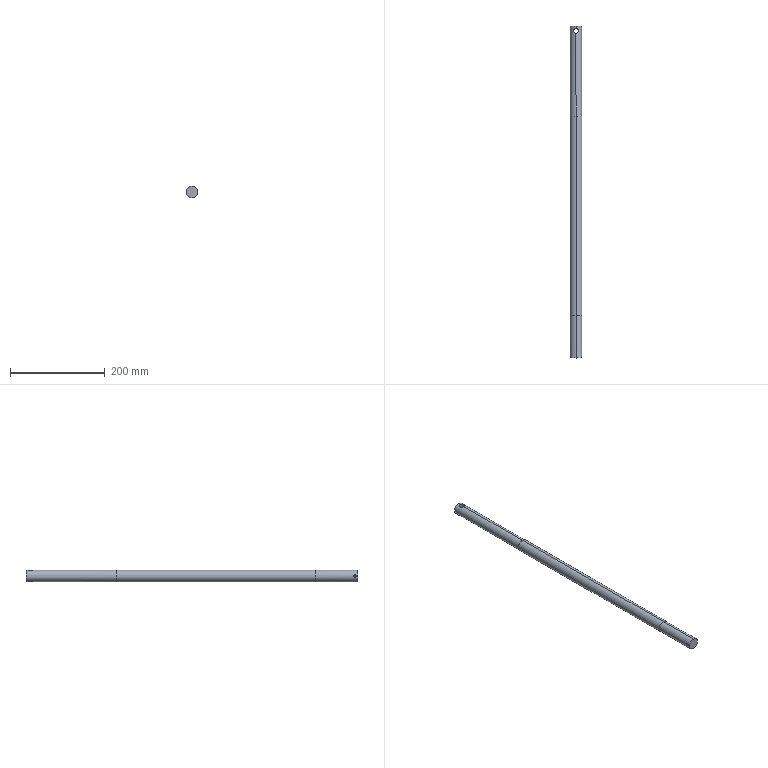Part | SolidWorks | features ICE 4, Extrusion 1 | 1 solid | 14 faces | box 25 x 700 x 25 mm | volume 330452 mm3 | cylinder 10 | plane 4 | commonest cylinder face diameters 24 x4 5 x2 10.2 x2 25 x2
STEP:
#1=CARTESIAN_POINT('',(-11.737,6.,2.5));
#2=VERTEX_POINT('',#1);
#3=CARTESIAN_POINT('',(-11.737,6.,-2.5));
#4=VERTEX_POINT('',#3);
#5=CARTESIAN_POINT('',(-11.737,6.,2.5));
#6=CARTESIAN_POINT('',(-11.737,5.673,2.5));
#7=CARTESIAN_POINT('',(-11.751,5.343,2.434));
#8=CARTESIAN_POINT('',(-11.788,4.892,2.247));
#9=CARTESIAN_POINT('',(-11.803,4.746,2.169));
#10=CARTESIAN_POINT('',(-11.835,4.474,1.987));
#11=CARTESIAN_POINT('',(-11.852,4.349,1.884));
#12=CARTESIAN_POINT('',(-11.886,4.118,1.654));
#13=CARTESIAN_POINT('',(-11.903,4.013,1.525));
#14=CARTESIAN_POINT('',(-11.935,3.832,1.255));
#15=CARTESIAN_POINT('',(-11.949,3.755,1.112));
#16=CARTESIAN_POINT('',(-11.986,3.565,0.6564));
#17=CARTESIAN_POINT('',(-12.,3.5,0.3312));
#18=CARTESIAN_POINT('',(-12.,3.5,-0.1639));
#19=CARTESIAN_POINT('',(-11.997,3.516,-0.3265));
#20=CARTESIAN_POINT('',(-11.984,3.58,-0.647));
#21=CARTESIAN_POINT('',(-11.974,3.628,-0.8064));
#22=CARTESIAN_POINT('',(-11.95,3.753,-1.108));
#23=CARTESIAN_POINT('',(-11.935,3.83,-1.252));
#24=CARTESIAN_POINT('',(-11.904,4.012,-1.524));
#25=CARTESIAN_POINT('',(-11.886,4.116,-1.652));
#26=CARTESIAN_POINT('',(-11.835,4.461,-1.997));
#27=CARTESIAN_POINT('',(-11.8,4.739,-2.183));
#28=CARTESIAN_POINT('',(-11.764,5.19,-2.371));
#29=CARTESIAN_POINT('',(-11.754,5.348,-2.419));
#30=CARTESIAN_POINT('',(-11.74,5.671,-2.484));
#31=CARTESIAN_POINT('',(-11.737,5.834,-2.5));
#32=CARTESIAN_POINT('',(-11.737,6.,-2.5));
#33=B_SPLINE_CURVE_WITH_KNOTS('',3,(#5,#6,#7,#8,#9,#10,#11,#12,#13,#14,#15,#16,#17,#18,#19,#20,#21,#22,#23,#24,#25,#26,#27,#28,#29,#30,#31,#32),.UNSPECIFIED.,.F.,.F.,(4,2,2,2,2,2,2,2,2,2,2,2,2,4),(0.007838,0.008817,0.009307,0.009797,0.01029,0.01078,0.01176,0.01225,0.01273,0.01322,0.01371,0.01469,0.01518,0.01567),.UNSPECIFIED.);
#34=EDGE_CURVE('',#2,#4,#33,.T.);
#35=ORIENTED_EDGE('',*,*,#34,.F.);
#36=CARTESIAN_POINT('',(11.737,6.,2.5));
#37=VERTEX_POINT('',#36);
#38=CARTESIAN_POINT('',(-12.5,6.,2.5));
#39=DIRECTION('',(1.,0.,0.));
#40=VECTOR('',#39,1000.);
#41=LINE('',#38,#40);
#42=EDGE_CURVE('',#2,#37,#41,.T.);
#43=ORIENTED_EDGE('',*,*,#42,.T.);
#44=CARTESIAN_POINT('',(11.737,6.,-2.5));
#45=VERTEX_POINT('',#44);
#46=CARTESIAN_POINT('',(11.737,6.,-2.5));
#47=CARTESIAN_POINT('',(11.737,5.834,-2.5));
#48=CARTESIAN_POINT('',(11.74,5.672,-2.484));
#49=CARTESIAN_POINT('',(11.754,5.351,-2.42));
#50=CARTESIAN_POINT('',(11.763,5.192,-2.372));
#51=CARTESIAN_POINT('',(11.788,4.89,-2.246));
#52=CARTESIAN_POINT('',(11.803,4.746,-2.169));
#53=CARTESIAN_POINT('',(11.835,4.475,-1.988));
#54=CARTESIAN_POINT('',(11.852,4.347,-1.882));
#55=CARTESIAN_POINT('',(11.903,4.002,-1.537));
#56=CARTESIAN_POINT('',(11.938,3.816,-1.259));
#57=CARTESIAN_POINT('',(11.974,3.629,-0.8081));
#58=CARTESIAN_POINT('',(11.983,3.58,-0.65));
#59=CARTESIAN_POINT('',(11.997,3.516,-0.3271));
#60=CARTESIAN_POINT('',(12.,3.5,-0.1645));
#61=CARTESIAN_POINT('',(12.,3.5,0.1626));
#62=CARTESIAN_POINT('',(11.997,3.516,0.3288));
#63=CARTESIAN_POINT('',(11.983,3.58,0.6498));
#64=CARTESIAN_POINT('',(11.974,3.628,0.8059));
#65=CARTESIAN_POINT('',(11.95,3.753,1.109));
#66=CARTESIAN_POINT('',(11.935,3.832,1.255));
#67=CARTESIAN_POINT('',(11.903,4.012,1.525));
#68=CARTESIAN_POINT('',(11.886,4.116,1.652));
#69=CARTESIAN_POINT('',(11.852,4.349,1.884));
#70=CARTESIAN_POINT('',(11.835,4.474,1.987));
#71=CARTESIAN_POINT('',(11.803,4.745,2.168));
#72=CARTESIAN_POINT('',(11.788,4.891,2.247));
#73=CARTESIAN_POINT('',(11.763,5.193,2.372));
#74=CARTESIAN_POINT('',(11.754,5.349,2.419));
#75=CARTESIAN_POINT('',(11.74,5.671,2.484));
#76=CARTESIAN_POINT('',(11.737,5.837,2.5));
#77=CARTESIAN_POINT('',(11.737,6.,2.5));
#78=B_SPLINE_CURVE_WITH_KNOTS('',3,(#46,#47,#48,#49,#50,#51,#52,#53,#54,#55,#56,#57,#58,#59,#60,#61,#62,#63,#64,#65,#66,#67,#68,#69,#70,#71,#72,#73,#74,#75,#76,#77),.UNSPECIFIED.,.F.,.F.,(4,2,2,2,2,2,2,2,2,2,2,2,2,2,2,4),(0.,0.0004899,0.0009797,0.00147,0.001959,0.002939,0.003429,0.003919,0.004409,0.004899,0.005388,0.005878,0.006368,0.006858,0.007348,0.007838),.UNSPECIFIED.);
#79=EDGE_CURVE('',#45,#37,#78,.T.);
#80=ORIENTED_EDGE('',*,*,#79,.F.);
#81=CARTESIAN_POINT('',(-12.5,6.,-2.5));
#82=DIRECTION('',(1.,0.,0.));
#83=VECTOR('',#82,1000.);
#84=LINE('',#81,#83);
#85=EDGE_CURVE('',#4,#45,#84,.T.);
#86=ORIENTED_EDGE('',*,*,#85,.F.);
#87=EDGE_LOOP('',(#35,#43,#80,#86));
#88=FACE_OUTER_BOUND('',#87,.T.);
#89=CARTESIAN_POINT('',(-12.5,6.,0.));
#90=DIRECTION('',(1.,0.,0.));
#91=DIRECTION('',(0.,0.,-1.));
#92=AXIS2_PLACEMENT_3D('',#89,#90,#91);
#93=CYLINDRICAL_SURFACE('',#92,2.5);
#94=ADVANCED_FACE('',(#88),#93,.F.);
#95=CARTESIAN_POINT('',(-5.1,690.,-10.862));
#96=VERTEX_POINT('',#95);
#97=CARTESIAN_POINT('',(0.,684.9,-12.));
#98=VERTEX_POINT('',#97);
#99=CARTESIAN_POINT('',(-5.1,690.,-10.862));
#100=CARTESIAN_POINT('',(-5.1,689.663,-10.862));
#101=CARTESIAN_POINT('',(-5.066,689.321,-10.879));
#102=CARTESIAN_POINT('',(-4.933,688.663,-10.939));
#103=CARTESIAN_POINT('',(-4.835,688.342,-10.984));
#104=CARTESIAN_POINT('',(-4.575,687.722,-11.094));
#105=CARTESIAN_POINT('',(-4.418,687.431,-11.159));
#106=CARTESIAN_POINT('',(-4.05,686.883,-11.298));
#107=CARTESIAN_POINT('',(-3.837,686.624,-11.373));
#108=CARTESIAN_POINT('',(-3.371,686.159,-11.519));
#109=CARTESIAN_POINT('',(-3.117,685.95,-11.591));
#110=CARTESIAN_POINT('',(-2.704,685.673,-11.692));
#111=CARTESIAN_POINT('',(-2.56,685.586,-11.725));
#112=CARTESIAN_POINT('',(-2.267,685.428,-11.785));
#113=CARTESIAN_POINT('',(-2.117,685.357,-11.813));
#114=CARTESIAN_POINT('',(-1.657,685.165,-11.889));
#115=CARTESIAN_POINT('',(-1.338,685.067,-11.93));
#116=CARTESIAN_POINT('',(-0.6717,684.933,-11.986));
#117=CARTESIAN_POINT('',(-0.3361,684.9,-12.));
#118=CARTESIAN_POINT('',(0.,684.9,-12.));
#119=B_SPLINE_CURVE_WITH_KNOTS('',3,(#99,#100,#101,#102,#103,#104,#105,#106,#107,#108,#109,#110,#111,#112,#113,#114,#115,#116,#117,#118),.UNSPECIFIED.,.F.,.F.,(4,2,2,2,2,2,2,2,2,4),(0.008073,0.009081,0.01009,0.0111,0.01211,0.01311,0.01362,0.01412,0.01513,0.01614),.UNSPECIFIED.);
#120=EDGE_CURVE('',#96,#98,#119,.T.);
#121=ORIENTED_EDGE('',*,*,#120,.F.);
#122=CARTESIAN_POINT('',(-5.1,690.,10.862));
#123=VERTEX_POINT('',#122);
#124=CARTESIAN_POINT('',(-5.1,690.,-12.5));
#125=DIRECTION('',(0.,0.,1.));
#126=VECTOR('',#125,1000.);
#127=LINE('',#124,#126);
#128=EDGE_CURVE('',#96,#123,#127,.T.);
#129=ORIENTED_EDGE('',*,*,#128,.T.);
#130=CARTESIAN_POINT('',(0.,684.9,12.));
#131=VERTEX_POINT('',#130);
#132=CARTESIAN_POINT('',(0.,684.9,12.));
#133=CARTESIAN_POINT('',(-0.3374,684.9,12.));
#134=CARTESIAN_POINT('',(-0.6794,684.934,11.985));
#135=CARTESIAN_POINT('',(-1.337,685.067,11.93));
#136=CARTESIAN_POINT('',(-1.659,685.166,11.889));
#137=CARTESIAN_POINT('',(-2.28,685.425,11.786));
#138=CARTESIAN_POINT('',(-2.571,685.583,11.725));
#139=CARTESIAN_POINT('',(-3.12,685.952,11.591));
#140=CARTESIAN_POINT('',(-3.379,686.166,11.517));
#141=CARTESIAN_POINT('',(-3.844,686.632,11.37));
#142=CARTESIAN_POINT('',(-4.052,686.886,11.297));
#143=CARTESIAN_POINT('',(-4.329,687.299,11.192));
#144=CARTESIAN_POINT('',(-4.415,687.442,11.158));
#145=CARTESIAN_POINT('',(-4.573,687.735,11.095));
#146=CARTESIAN_POINT('',(-4.644,687.885,11.065));
#147=CARTESIAN_POINT('',(-4.835,688.344,10.984));
#148=CARTESIAN_POINT('',(-4.933,688.662,10.939));
#149=CARTESIAN_POINT('',(-5.067,689.328,10.878));
#150=CARTESIAN_POINT('',(-5.1,689.664,10.862));
#151=CARTESIAN_POINT('',(-5.1,690.,10.862));
#152=B_SPLINE_CURVE_WITH_KNOTS('',3,(#132,#133,#134,#135,#136,#137,#138,#139,#140,#141,#142,#143,#144,#145,#146,#147,#148,#149,#150,#151),.UNSPECIFIED.,.F.,.F.,(4,2,2,2,2,2,2,2,2,4),(0.008072,0.00908,0.01009,0.0111,0.01211,0.01311,0.01362,0.01412,0.01513,0.01614),.UNSPECIFIED.);
#153=EDGE_CURVE('',#131,#123,#152,.T.);
#154=ORIENTED_EDGE('',*,*,#153,.F.);
#155=CARTESIAN_POINT('',(5.1,690.,10.862));
#156=VERTEX_POINT('',#155);
#157=CARTESIAN_POINT('',(5.1,690.,10.862));
#158=CARTESIAN_POINT('',(5.1,689.658,10.862));
#159=CARTESIAN_POINT('',(5.066,689.324,10.878));
#160=CARTESIAN_POINT('',(4.934,688.666,10.939));
#161=CARTESIAN_POINT('',(4.834,688.34,10.984));
#162=CARTESIAN_POINT('',(4.577,687.725,11.094));
#163=CARTESIAN_POINT('',(4.42,687.434,11.158));
#164=CARTESIAN_POINT('',(4.05,686.882,11.298));
#165=CARTESIAN_POINT('',(3.838,686.625,11.372));
#166=CARTESIAN_POINT('',(3.373,686.161,11.519));
#167=CARTESIAN_POINT('',(3.117,685.95,11.592));
#168=CARTESIAN_POINT('',(2.563,685.578,11.727));
#169=CARTESIAN_POINT('',(2.272,685.422,11.787));
#170=CARTESIAN_POINT('',(1.812,685.23,11.863));
#171=CARTESIAN_POINT('',(1.655,685.173,11.886));
#172=CARTESIAN_POINT('',(1.333,685.074,11.927));
#173=CARTESIAN_POINT('',(1.167,685.033,11.944));
#174=CARTESIAN_POINT('',(0.6717,684.933,11.986));
#175=CARTESIAN_POINT('',(0.3377,684.9,12.));
#176=CARTESIAN_POINT('',(0.,684.9,12.));
#177=B_SPLINE_CURVE_WITH_KNOTS('',3,(#157,#158,#159,#160,#161,#162,#163,#164,#165,#166,#167,#168,#169,#170,#171,#172,#173,#174,#175,#176),.UNSPECIFIED.,.F.,.F.,(4,2,2,2,2,2,2,2,2,4),(0.,0.001009,0.002018,0.003027,0.004036,0.005045,0.006054,0.006558,0.007063,0.008072),.UNSPECIFIED.);
#178=EDGE_CURVE('',#156,#131,#177,.T.);
#179=ORIENTED_EDGE('',*,*,#178,.F.);
#180=CARTESIAN_POINT('',(5.1,690.,-10.862));
#181=VERTEX_POINT('',#180);
#182=CARTESIAN_POINT('',(5.1,690.,-12.5));
#183=DIRECTION('',(0.,0.,1.));
#184=VECTOR('',#183,1000.);
#185=LINE('',#182,#184);
#186=EDGE_CURVE('',#181,#156,#185,.T.);
#187=ORIENTED_EDGE('',*,*,#186,.F.);
#188=CARTESIAN_POINT('',(0.,684.9,-12.));
#189=CARTESIAN_POINT('',(0.168,684.9,-12.));
#190=CARTESIAN_POINT('',(0.3363,684.908,-11.996));
#191=CARTESIAN_POINT('',(0.6735,684.942,-11.982));
#192=CARTESIAN_POINT('',(0.8425,684.967,-11.972));
#193=CARTESIAN_POINT('',(1.338,685.067,-11.93));
#194=CARTESIAN_POINT('',(1.658,685.165,-11.889));
#195=CARTESIAN_POINT('',(2.121,685.359,-11.812));
#196=CARTESIAN_POINT('',(2.273,685.432,-11.784));
#197=CARTESIAN_POINT('',(2.567,685.59,-11.723));
#198=CARTESIAN_POINT('',(2.708,685.676,-11.691));
#199=CARTESIAN_POINT('',(3.119,685.952,-11.591));
#200=CARTESIAN_POINT('',(3.376,686.163,-11.518));
#201=CARTESIAN_POINT('',(3.844,686.632,-11.37));
#202=CARTESIAN_POINT('',(4.053,686.886,-11.297));
#203=CARTESIAN_POINT('',(4.419,687.434,-11.158));
#204=CARTESIAN_POINT('',(4.579,687.731,-11.093));
#205=CARTESIAN_POINT('',(4.835,688.345,-10.984));
#206=CARTESIAN_POINT('',(4.933,688.663,-10.939));
#207=CARTESIAN_POINT('',(5.066,689.322,-10.879));
#208=CARTESIAN_POINT('',(5.1,689.664,-10.862));
#209=CARTESIAN_POINT('',(5.1,690.,-10.862));
#210=B_SPLINE_CURVE_WITH_KNOTS('',3,(#188,#189,#190,#191,#192,#193,#194,#195,#196,#197,#198,#199,#200,#201,#202,#203,#204,#205,#206,#207,#208,#209),.UNSPECIFIED.,.F.,.F.,(4,2,2,2,2,2,2,2,2,2,4),(0.01614,0.01664,0.01715,0.01816,0.01866,0.01916,0.02017,0.02118,0.02219,0.0232,0.0242),.UNSPECIFIED.);
#211=EDGE_CURVE('',#98,#181,#210,.T.);
#212=ORIENTED_EDGE('',*,*,#211,.F.);
#213=EDGE_LOOP('',(#121,#129,#154,#179,#187,#212));
#214=FACE_OUTER_BOUND('',#213,.T.);
#215=CARTESIAN_POINT('',(0.,690.,-12.5));
#216=DIRECTION('',(0.,0.,1.));
#217=DIRECTION('',(1.,0.,0.));
#218=AXIS2_PLACEMENT_3D('',#215,#216,#217);
#219=CYLINDRICAL_SURFACE('',#218,5.1);
#220=ADVANCED_FACE('',(#214),#219,.F.);
#221=CARTESIAN_POINT('',(0.,700.,12.));
#222=VERTEX_POINT('',#221);
#223=CARTESIAN_POINT('',(0.,700.,-12.));
#224=VERTEX_POINT('',#223);
#225=CARTESIAN_POINT('',(0.,700.,0.));
#226=DIRECTION('',(0.,1.,0.));
#227=DIRECTION('',(0.,0.,1.));
#228=AXIS2_PLACEMENT_3D('',#225,#226,#227);
#229=CIRCLE('',#228,12.);
#230=EDGE_CURVE('',#222,#224,#229,.T.);
#231=ORIENTED_EDGE('',*,*,#230,.F.);
#232=CARTESIAN_POINT('',(0.,695.1,12.));
#233=VERTEX_POINT('',#232);
#234=CARTESIAN_POINT('',(0.,700.,12.));
#235=DIRECTION('',(0.,-1.,0.));
#236=VECTOR('',#235,1000.);
#237=LINE('',#234,#236);
#238=EDGE_CURVE('',#222,#233,#237,.T.);
#239=ORIENTED_EDGE('',*,*,#238,.T.);
#240=CARTESIAN_POINT('',(0.,695.1,12.));
#241=CARTESIAN_POINT('',(0.3362,695.1,12.));
#242=CARTESIAN_POINT('',(0.6715,695.067,11.986));
#243=CARTESIAN_POINT('',(1.338,694.933,11.93));
#244=CARTESIAN_POINT('',(1.658,694.835,11.889));
#245=CARTESIAN_POINT('',(2.273,694.578,11.787));
#246=CARTESIAN_POINT('',(2.57,694.417,11.725));
#247=CARTESIAN_POINT('',(3.119,694.048,11.591));
#248=CARTESIAN_POINT('',(3.373,693.839,11.519));
#249=CARTESIAN_POINT('',(3.842,693.371,11.371));
#250=CARTESIAN_POINT('',(4.053,693.114,11.297));
#251=CARTESIAN_POINT('',(4.419,692.567,11.158));
#252=CARTESIAN_POINT('',(4.577,692.275,11.094));
#253=CARTESIAN_POINT('',(4.836,691.655,10.983));
#254=CARTESIAN_POINT('',(4.933,691.336,10.939));
#255=CARTESIAN_POINT('',(5.065,690.681,10.879));
#256=CARTESIAN_POINT('',(5.1,690.341,10.862));
#257=CARTESIAN_POINT('',(5.1,690.,10.862));
#258=B_SPLINE_CURVE_WITH_KNOTS('',3,(#240,#241,#242,#243,#244,#245,#246,#247,#248,#249,#250,#251,#252,#253,#254,#255,#256,#257),.UNSPECIFIED.,.F.,.F.,(4,2,2,2,2,2,2,2,4),(0.0242,0.02521,0.02622,0.02722,0.02823,0.02924,0.03025,0.03125,0.03226),.UNSPECIFIED.);
#259=EDGE_CURVE('',#233,#156,#258,.T.);
#260=ORIENTED_EDGE('',*,*,#259,.T.);
#261=ORIENTED_EDGE('',*,*,#178,.T.);
#262=CARTESIAN_POINT('',(0.,510.,12.));
#263=VERTEX_POINT('',#262);
#264=CARTESIAN_POINT('',(0.,700.,12.));
#265=DIRECTION('',(0.,-1.,0.));
#266=VECTOR('',#265,1000.);
#267=LINE('',#264,#266);
#268=EDGE_CURVE('',#131,#263,#267,.T.);
#269=ORIENTED_EDGE('',*,*,#268,.T.);
#270=CARTESIAN_POINT('',(0.,510.,-12.));
#271=VERTEX_POINT('',#270);
#272=CARTESIAN_POINT('',(0.,510.,0.));
#273=DIRECTION('',(0.,1.,0.));
#274=DIRECTION('',(0.,0.,1.));
#275=AXIS2_PLACEMENT_3D('',#272,#273,#274);
#276=CIRCLE('',#275,12.);
#277=EDGE_CURVE('',#263,#271,#276,.T.);
#278=ORIENTED_EDGE('',*,*,#277,.T.);
#279=CARTESIAN_POINT('',(0.,700.,-12.));
#280=DIRECTION('',(0.,-1.,0.));
#281=VECTOR('',#280,1000.);
#282=LINE('',#279,#281);
#283=EDGE_CURVE('',#98,#271,#282,.T.);
#284=ORIENTED_EDGE('',*,*,#283,.F.);
#285=ORIENTED_EDGE('',*,*,#211,.T.);
#286=CARTESIAN_POINT('',(0.,695.1,-12.));
#287=VERTEX_POINT('',#286);
#288=CARTESIAN_POINT('',(5.1,690.,-10.862));
#289=CARTESIAN_POINT('',(5.1,690.336,-10.862));
#290=CARTESIAN_POINT('',(5.067,690.671,-10.878));
#291=CARTESIAN_POINT('',(4.933,691.337,-10.939));
#292=CARTESIAN_POINT('',(4.835,691.657,-10.984));
#293=CARTESIAN_POINT('',(4.579,692.271,-11.093));
#294=CARTESIAN_POINT('',(4.419,692.568,-11.159));
#295=CARTESIAN_POINT('',(4.051,693.116,-11.297));
#296=CARTESIAN_POINT('',(3.842,693.37,-11.371));
#297=CARTESIAN_POINT('',(3.374,693.839,-11.519));
#298=CARTESIAN_POINT('',(3.117,694.05,-11.592));
#299=CARTESIAN_POINT('',(2.57,694.417,-11.725));
#300=CARTESIAN_POINT('',(2.277,694.576,-11.786));
#301=CARTESIAN_POINT('',(1.656,694.835,-11.889));
#302=CARTESIAN_POINT('',(1.337,694.933,-11.93));
#303=CARTESIAN_POINT('',(0.681,695.065,-11.985));
#304=CARTESIAN_POINT('',(0.341,695.1,-12.));
#305=CARTESIAN_POINT('',(0.,695.1,-12.));
#306=B_SPLINE_CURVE_WITH_KNOTS('',3,(#288,#289,#290,#291,#292,#293,#294,#295,#296,#297,#298,#299,#300,#301,#302,#303,#304,#305),.UNSPECIFIED.,.F.,.F.,(4,2,2,2,2,2,2,2,4),(0.0242,0.02521,0.02622,0.02723,0.02823,0.02924,0.03025,0.03126,0.03226),.UNSPECIFIED.);
#307=EDGE_CURVE('',#181,#287,#306,.T.);
#308=ORIENTED_EDGE('',*,*,#307,.T.);
#309=CARTESIAN_POINT('',(0.,700.,-12.));
#310=DIRECTION('',(0.,-1.,0.));
#311=VECTOR('',#310,1000.);
#312=LINE('',#309,#311);
#313=EDGE_CURVE('',#224,#287,#312,.T.);
#314=ORIENTED_EDGE('',*,*,#313,.F.);
#315=EDGE_LOOP('',(#231,#239,#260,#261,#269,#278,#284,#285,#308,#314));
#316=FACE_OUTER_BOUND('',#315,.T.);
#317=CARTESIAN_POINT('',(0.,700.,0.));
#318=DIRECTION('',(0.,-1.,0.));
#319=DIRECTION('',(0.,0.,-1.));
#320=AXIS2_PLACEMENT_3D('',#317,#318,#319);
#321=CYLINDRICAL_SURFACE('',#320,12.);
#322=ADVANCED_FACE('',(#316),#321,.T.);
#323=CARTESIAN_POINT('',(0.,510.,12.5));
#324=VERTEX_POINT('',#323);
#325=CARTESIAN_POINT('',(0.,510.,-12.5));
#326=VERTEX_POINT('',#325);
#327=CARTESIAN_POINT('',(0.,510.,0.));
#328=DIRECTION('',(0.,1.,0.));
#329=DIRECTION('',(0.,0.,1.));
#330=AXIS2_PLACEMENT_3D('',#327,#328,#329);
#331=CIRCLE('',#330,12.5);
#332=EDGE_CURVE('',#324,#326,#331,.T.);
#333=ORIENTED_EDGE('',*,*,#332,.F.);
#334=CARTESIAN_POINT('',(0.,90.,12.5));
#335=VERTEX_POINT('',#334);
#336=CARTESIAN_POINT('',(0.,510.,12.5));
#337=DIRECTION('',(0.,-1.,0.));
#338=VECTOR('',#337,1000.);
#339=LINE('',#336,#338);
#340=EDGE_CURVE('',#324,#335,#339,.T.);
#341=ORIENTED_EDGE('',*,*,#340,.T.);
#342=CARTESIAN_POINT('',(0.,90.,-12.5));
#343=VERTEX_POINT('',#342);
#344=CARTESIAN_POINT('',(0.,90.,0.));
#345=DIRECTION('',(0.,1.,0.));
#346=DIRECTION('',(0.,0.,1.));
#347=AXIS2_PLACEMENT_3D('',#344,#345,#346);
#348=CIRCLE('',#347,12.5);
#349=EDGE_CURVE('',#335,#343,#348,.T.);
#350=ORIENTED_EDGE('',*,*,#349,.T.);
#351=CARTESIAN_POINT('',(0.,510.,-12.5));
#352=DIRECTION('',(0.,-1.,0.));
#353=VECTOR('',#352,1000.);
#354=LINE('',#351,#353);
#355=EDGE_CURVE('',#326,#343,#354,.T.);
#356=ORIENTED_EDGE('',*,*,#355,.F.);
#357=EDGE_LOOP('',(#333,#341,#350,#356));
#358=FACE_OUTER_BOUND('',#357,.T.);
#359=CARTESIAN_POINT('',(0.,510.,0.));
#360=DIRECTION('',(0.,-1.,0.));
#361=DIRECTION('',(0.,0.,-1.));
#362=AXIS2_PLACEMENT_3D('',#359,#360,#361);
#363=CYLINDRICAL_SURFACE('',#362,12.5);
#364=ADVANCED_FACE('',(#358),#363,.T.);
#365=ORIENTED_EDGE('',*,*,#79,.T.);
#366=CARTESIAN_POINT('',(11.737,6.,2.5));
#367=CARTESIAN_POINT('',(11.737,6.327,2.5));
#368=CARTESIAN_POINT('',(11.751,6.657,2.434));
#369=CARTESIAN_POINT('',(11.788,7.108,2.247));
#370=CARTESIAN_POINT('',(11.803,7.254,2.169));
#371=CARTESIAN_POINT('',(11.835,7.526,1.987));
#372=CARTESIAN_POINT('',(11.852,7.651,1.884));
#373=CARTESIAN_POINT('',(11.886,7.882,1.654));
#374=CARTESIAN_POINT('',(11.903,7.987,1.525));
#375=CARTESIAN_POINT('',(11.935,8.168,1.255));
#376=CARTESIAN_POINT('',(11.949,8.245,1.112));
#377=CARTESIAN_POINT('',(11.986,8.435,0.6564));
#378=CARTESIAN_POINT('',(12.,8.5,0.3312));
#379=CARTESIAN_POINT('',(12.,8.5,-0.1639));
#380=CARTESIAN_POINT('',(11.997,8.484,-0.3265));
#381=CARTESIAN_POINT('',(11.984,8.42,-0.647));
#382=CARTESIAN_POINT('',(11.974,8.372,-0.8064));
#383=CARTESIAN_POINT('',(11.95,8.247,-1.108));
#384=CARTESIAN_POINT('',(11.935,8.17,-1.252));
#385=CARTESIAN_POINT('',(11.904,7.988,-1.524));
#386=CARTESIAN_POINT('',(11.886,7.884,-1.652));
#387=CARTESIAN_POINT('',(11.835,7.539,-1.997));
#388=CARTESIAN_POINT('',(11.8,7.261,-2.183));
#389=CARTESIAN_POINT('',(11.764,6.81,-2.371));
#390=CARTESIAN_POINT('',(11.754,6.652,-2.419));
#391=CARTESIAN_POINT('',(11.74,6.329,-2.484));
#392=CARTESIAN_POINT('',(11.737,6.166,-2.5));
#393=CARTESIAN_POINT('',(11.737,6.,-2.5));
#394=B_SPLINE_CURVE_WITH_KNOTS('',3,(#366,#367,#368,#369,#370,#371,#372,#373,#374,#375,#376,#377,#378,#379,#380,#381,#382,#383,#384,#385,#386,#387,#388,#389,#390,#391,#392,#393),.UNSPECIFIED.,.F.,.F.,(4,2,2,2,2,2,2,2,2,2,2,2,2,4),(0.007838,0.008817,0.009307,0.009797,0.01029,0.01078,0.01176,0.01225,0.01273,0.01322,0.01371,0.01469,0.01518,0.01567),.UNSPECIFIED.);
#395=EDGE_CURVE('',#37,#45,#394,.T.);
#396=ORIENTED_EDGE('',*,*,#395,.T.);
#397=EDGE_LOOP('',(#365,#396));
#398=FACE_BOUND('',#397,.T.);
#399=CARTESIAN_POINT('',(0.,90.,12.));
#400=VERTEX_POINT('',#399);
#401=CARTESIAN_POINT('',(0.,90.,-12.));
#402=VERTEX_POINT('',#401);
#403=CARTESIAN_POINT('',(0.,90.,0.));
#404=DIRECTION('',(0.,1.,0.));
#405=DIRECTION('',(0.,0.,1.));
#406=AXIS2_PLACEMENT_3D('',#403,#404,#405);
#407=CIRCLE('',#406,12.);
#408=EDGE_CURVE('',#400,#402,#407,.T.);
#409=ORIENTED_EDGE('',*,*,#408,.F.);
#410=CARTESIAN_POINT('',(0.,0.,12.));
#411=VERTEX_POINT('',#410);
#412=CARTESIAN_POINT('',(0.,90.,12.));
#413=DIRECTION('',(0.,-1.,0.));
#414=VECTOR('',#413,1000.);
#415=LINE('',#412,#414);
#416=EDGE_CURVE('',#400,#411,#415,.T.);
#417=ORIENTED_EDGE('',*,*,#416,.T.);
#418=CARTESIAN_POINT('',(0.,0.,-12.));
#419=VERTEX_POINT('',#418);
#420=CARTESIAN_POINT('',(0.,0.,0.));
#421=DIRECTION('',(0.,1.,0.));
#422=DIRECTION('',(0.,0.,1.));
#423=AXIS2_PLACEMENT_3D('',#420,#421,#422);
#424=CIRCLE('',#423,12.);
#425=EDGE_CURVE('',#411,#419,#424,.T.);
#426=ORIENTED_EDGE('',*,*,#425,.T.);
#427=CARTESIAN_POINT('',(0.,90.,-12.));
#428=DIRECTION('',(0.,-1.,0.));
#429=VECTOR('',#428,1000.);
#430=LINE('',#427,#429);
#431=EDGE_CURVE('',#402,#419,#430,.T.);
#432=ORIENTED_EDGE('',*,*,#431,.F.);
#433=EDGE_LOOP('',(#409,#417,#426,#432));
#434=FACE_OUTER_BOUND('',#433,.T.);
#435=CARTESIAN_POINT('',(0.,90.,0.));
#436=DIRECTION('',(0.,-1.,0.));
#437=DIRECTION('',(0.,0.,-1.));
#438=AXIS2_PLACEMENT_3D('',#435,#436,#437);
#439=CYLINDRICAL_SURFACE('',#438,12.);
#440=ADVANCED_FACE('',(#398,#434),#439,.T.);
#441=ORIENTED_EDGE('',*,*,#416,.F.);
#442=CARTESIAN_POINT('',(0.,90.,0.));
#443=DIRECTION('',(0.,1.,0.));
#444=DIRECTION('',(0.,0.,1.));
#445=AXIS2_PLACEMENT_3D('',#442,#443,#444);
#446=CIRCLE('',#445,12.);
#447=EDGE_CURVE('',#402,#400,#446,.T.);
#448=ORIENTED_EDGE('',*,*,#447,.F.);
#449=ORIENTED_EDGE('',*,*,#431,.T.);
#450=CARTESIAN_POINT('',(0.,0.,0.));
#451=DIRECTION('',(0.,1.,0.));
#452=DIRECTION('',(0.,0.,1.));
#453=AXIS2_PLACEMENT_3D('',#450,#451,#452);
#454=CIRCLE('',#453,12.);
#455=EDGE_CURVE('',#419,#411,#454,.T.);
#456=ORIENTED_EDGE('',*,*,#455,.T.);
#457=EDGE_LOOP('',(#441,#448,#449,#456));
#458=FACE_OUTER_BOUND('',#457,.T.);
#459=CARTESIAN_POINT('',(-11.737,6.,-2.5));
#460=CARTESIAN_POINT('',(-11.737,6.166,-2.5));
#461=CARTESIAN_POINT('',(-11.74,6.328,-2.484));
#462=CARTESIAN_POINT('',(-11.754,6.649,-2.42));
#463=CARTESIAN_POINT('',(-11.763,6.808,-2.372));
#464=CARTESIAN_POINT('',(-11.788,7.11,-2.246));
#465=CARTESIAN_POINT('',(-11.803,7.254,-2.169));
#466=CARTESIAN_POINT('',(-11.835,7.525,-1.988));
#467=CARTESIAN_POINT('',(-11.852,7.653,-1.882));
#468=CARTESIAN_POINT('',(-11.903,7.998,-1.537));
#469=CARTESIAN_POINT('',(-11.938,8.184,-1.259));
#470=CARTESIAN_POINT('',(-11.974,8.371,-0.8081));
#471=CARTESIAN_POINT('',(-11.983,8.42,-0.65));
#472=CARTESIAN_POINT('',(-11.997,8.484,-0.3271));
#473=CARTESIAN_POINT('',(-12.,8.5,-0.1645));
#474=CARTESIAN_POINT('',(-12.,8.5,0.1626));
#475=CARTESIAN_POINT('',(-11.997,8.484,0.3288));
#476=CARTESIAN_POINT('',(-11.983,8.42,0.6498));
#477=CARTESIAN_POINT('',(-11.974,8.372,0.8059));
#478=CARTESIAN_POINT('',(-11.95,8.247,1.109));
#479=CARTESIAN_POINT('',(-11.935,8.168,1.255));
#480=CARTESIAN_POINT('',(-11.903,7.988,1.525));
#481=CARTESIAN_POINT('',(-11.886,7.884,1.652));
#482=CARTESIAN_POINT('',(-11.852,7.651,1.884));
#483=CARTESIAN_POINT('',(-11.835,7.526,1.987));
#484=CARTESIAN_POINT('',(-11.803,7.255,2.168));
#485=CARTESIAN_POINT('',(-11.788,7.109,2.247));
#486=CARTESIAN_POINT('',(-11.763,6.807,2.372));
#487=CARTESIAN_POINT('',(-11.754,6.651,2.419));
#488=CARTESIAN_POINT('',(-11.74,6.329,2.484));
#489=CARTESIAN_POINT('',(-11.737,6.163,2.5));
#490=CARTESIAN_POINT('',(-11.737,6.,2.5));
#491=B_SPLINE_CURVE_WITH_KNOTS('',3,(#459,#460,#461,#462,#463,#464,#465,#466,#467,#468,#469,#470,#471,#472,#473,#474,#475,#476,#477,#478,#479,#480,#481,#482,#483,#484,#485,#486,#487,#488,#489,#490),.UNSPECIFIED.,.F.,.F.,(4,2,2,2,2,2,2,2,2,2,2,2,2,2,2,4),(0.,0.0004899,0.0009797,0.00147,0.001959,0.002939,0.003429,0.003919,0.004409,0.004899,0.005388,0.005878,0.006368,0.006858,0.007348,0.007838),.UNSPECIFIED.);
#492=EDGE_CURVE('',#4,#2,#491,.T.);
#493=ORIENTED_EDGE('',*,*,#492,.T.);
#494=ORIENTED_EDGE('',*,*,#34,.T.);
#495=EDGE_LOOP('',(#493,#494));
#496=FACE_BOUND('',#495,.T.);
#497=CARTESIAN_POINT('',(0.,90.,0.));
#498=DIRECTION('',(0.,-1.,0.));
#499=DIRECTION('',(0.,0.,-1.));
#500=AXIS2_PLACEMENT_3D('',#497,#498,#499);
#501=CYLINDRICAL_SURFACE('',#500,12.);
#502=ADVANCED_FACE('',(#458,#496),#501,.T.);
#503=ORIENTED_EDGE('',*,*,#455,.F.);
#504=ORIENTED_EDGE('',*,*,#425,.F.);
#505=EDGE_LOOP('',(#503,#504));
#506=FACE_OUTER_BOUND('',#505,.T.);
#507=CARTESIAN_POINT('',(0.,0.,0.));
#508=DIRECTION('',(0.,1.,0.));
#509=DIRECTION('',(0.,0.,1.));
#510=AXIS2_PLACEMENT_3D('',#507,#508,#509);
#511=PLANE('',#510);
#512=ADVANCED_FACE('',(#506),#511,.F.);
#513=ORIENTED_EDGE('',*,*,#340,.F.);
#514=CARTESIAN_POINT('',(0.,510.,0.));
#515=DIRECTION('',(0.,1.,0.));
#516=DIRECTION('',(0.,0.,1.));
#517=AXIS2_PLACEMENT_3D('',#514,#515,#516);
#518=CIRCLE('',#517,12.5);
#519=EDGE_CURVE('',#326,#324,#518,.T.);
#520=ORIENTED_EDGE('',*,*,#519,.F.);
#521=ORIENTED_EDGE('',*,*,#355,.T.);
#522=CARTESIAN_POINT('',(0.,90.,0.));
#523=DIRECTION('',(0.,1.,0.));
#524=DIRECTION('',(0.,0.,1.));
#525=AXIS2_PLACEMENT_3D('',#522,#523,#524);
#526=CIRCLE('',#525,12.5);
#527=EDGE_CURVE('',#343,#335,#526,.T.);
#528=ORIENTED_EDGE('',*,*,#527,.T.);
#529=EDGE_LOOP('',(#513,#520,#521,#528));
#530=FACE_OUTER_BOUND('',#529,.T.);
#531=CARTESIAN_POINT('',(0.,510.,0.));
#532=DIRECTION('',(0.,-1.,0.));
#533=DIRECTION('',(0.,0.,-1.));
#534=AXIS2_PLACEMENT_3D('',#531,#532,#533);
#535=CYLINDRICAL_SURFACE('',#534,12.5);
#536=ADVANCED_FACE('',(#530),#535,.T.);
#537=CARTESIAN_POINT('',(0.,510.,0.));
#538=DIRECTION('',(0.,1.,0.));
#539=DIRECTION('',(0.,0.,1.));
#540=AXIS2_PLACEMENT_3D('',#537,#538,#539);
#541=CIRCLE('',#540,12.);
#542=EDGE_CURVE('',#271,#263,#541,.T.);
#543=ORIENTED_EDGE('',*,*,#542,.F.);
#544=ORIENTED_EDGE('',*,*,#277,.F.);
#545=EDGE_LOOP('',(#543,#544));
#546=FACE_BOUND('',#545,.T.);
#547=ORIENTED_EDGE('',*,*,#519,.T.);
#548=ORIENTED_EDGE('',*,*,#332,.T.);
#549=EDGE_LOOP('',(#547,#548));
#550=FACE_OUTER_BOUND('',#549,.T.);
#551=CARTESIAN_POINT('',(0.,510.,0.));
#552=DIRECTION('',(0.,1.,0.));
#553=DIRECTION('',(0.,0.,1.));
#554=AXIS2_PLACEMENT_3D('',#551,#552,#553);
#555=PLANE('',#554);
#556=ADVANCED_FACE('',(#546,#550),#555,.T.);
#557=ORIENTED_EDGE('',*,*,#447,.T.);
#558=ORIENTED_EDGE('',*,*,#408,.T.);
#559=EDGE_LOOP('',(#557,#558));
#560=FACE_BOUND('',#559,.T.);
#561=ORIENTED_EDGE('',*,*,#527,.F.);
#562=ORIENTED_EDGE('',*,*,#349,.F.);
#563=EDGE_LOOP('',(#561,#562));
#564=FACE_OUTER_BOUND('',#563,.T.);
#565=CARTESIAN_POINT('',(0.,90.,0.));
#566=DIRECTION('',(0.,1.,0.));
#567=DIRECTION('',(0.,0.,1.));
#568=AXIS2_PLACEMENT_3D('',#565,#566,#567);
#569=PLANE('',#568);
#570=ADVANCED_FACE('',(#560,#564),#569,.F.);
#571=ORIENTED_EDGE('',*,*,#238,.F.);
#572=CARTESIAN_POINT('',(0.,700.,0.));
#573=DIRECTION('',(0.,1.,0.));
#574=DIRECTION('',(0.,0.,1.));
#575=AXIS2_PLACEMENT_3D('',#572,#573,#574);
#576=CIRCLE('',#575,12.);
#577=EDGE_CURVE('',#224,#222,#576,.T.);
#578=ORIENTED_EDGE('',*,*,#577,.F.);
#579=ORIENTED_EDGE('',*,*,#313,.T.);
#580=CARTESIAN_POINT('',(0.,695.1,-12.));
#581=CARTESIAN_POINT('',(-0.3415,695.1,-12.));
#582=CARTESIAN_POINT('',(-0.6765,695.066,-11.985));
#583=CARTESIAN_POINT('',(-1.334,694.934,-11.93));
#584=CARTESIAN_POINT('',(-1.661,694.834,-11.889));
#585=CARTESIAN_POINT('',(-2.277,694.576,-11.786));
#586=CARTESIAN_POINT('',(-2.569,694.418,-11.725));
#587=CARTESIAN_POINT('',(-3.12,694.048,-11.591));
#588=CARTESIAN_POINT('',(-3.378,693.835,-11.517));
#589=CARTESIAN_POINT('',(-3.842,693.37,-11.371));
#590=CARTESIAN_POINT('',(-4.053,693.114,-11.297));
#591=CARTESIAN_POINT('',(-4.423,692.561,-11.157));
#592=CARTESIAN_POINT('',(-4.579,692.269,-11.093));
#593=CARTESIAN_POINT('',(-4.771,691.81,-11.011));
#594=CARTESIAN_POINT('',(-4.827,691.653,-10.986));
#595=CARTESIAN_POINT('',(-4.926,691.332,-10.943));
#596=CARTESIAN_POINT('',(-4.968,691.167,-10.924));
#597=CARTESIAN_POINT('',(-5.067,690.671,-10.878));
#598=CARTESIAN_POINT('',(-5.1,690.337,-10.862));
#599=CARTESIAN_POINT('',(-5.1,690.,-10.862));
#600=B_SPLINE_CURVE_WITH_KNOTS('',3,(#580,#581,#582,#583,#584,#585,#586,#587,#588,#589,#590,#591,#592,#593,#594,#595,#596,#597,#598,#599),.UNSPECIFIED.,.F.,.F.,(4,2,2,2,2,2,2,2,2,4),(0.,0.001009,0.002018,0.003027,0.004037,0.005046,0.006055,0.006559,0.007064,0.008073),.UNSPECIFIED.);
#601=EDGE_CURVE('',#287,#96,#600,.T.);
#602=ORIENTED_EDGE('',*,*,#601,.T.);
#603=ORIENTED_EDGE('',*,*,#120,.T.);
#604=ORIENTED_EDGE('',*,*,#283,.T.);
#605=ORIENTED_EDGE('',*,*,#542,.T.);
#606=ORIENTED_EDGE('',*,*,#268,.F.);
#607=ORIENTED_EDGE('',*,*,#153,.T.);
#608=CARTESIAN_POINT('',(-5.1,690.,10.862));
#609=CARTESIAN_POINT('',(-5.1,690.168,10.862));
#610=CARTESIAN_POINT('',(-5.092,690.336,10.866));
#611=CARTESIAN_POINT('',(-5.058,690.673,10.882));
#612=CARTESIAN_POINT('',(-5.033,690.842,10.894));
#613=CARTESIAN_POINT('',(-4.933,691.338,10.939));
#614=CARTESIAN_POINT('',(-4.835,691.657,10.984));
#615=CARTESIAN_POINT('',(-4.642,692.119,11.066));
#616=CARTESIAN_POINT('',(-4.569,692.272,11.096));
#617=CARTESIAN_POINT('',(-4.411,692.564,11.16));
#618=CARTESIAN_POINT('',(-4.326,692.706,11.194));
#619=CARTESIAN_POINT('',(-4.05,693.117,11.297));
#620=CARTESIAN_POINT('',(-3.839,693.373,11.372));
#621=CARTESIAN_POINT('',(-3.371,693.842,11.519));
#622=CARTESIAN_POINT('',(-3.117,694.05,11.592));
#623=CARTESIAN_POINT('',(-2.569,694.418,11.725));
#624=CARTESIAN_POINT('',(-2.271,694.578,11.787));
#625=CARTESIAN_POINT('',(-1.656,694.835,11.889));
#626=CARTESIAN_POINT('',(-1.338,694.933,11.93));
#627=CARTESIAN_POINT('',(-0.8432,695.033,11.971));
#628=CARTESIAN_POINT('',(-0.6743,695.058,11.982));
#629=CARTESIAN_POINT('',(-0.3367,695.092,11.996));
#630=CARTESIAN_POINT('',(-0.1682,695.1,12.));
#631=CARTESIAN_POINT('',(0.,695.1,12.));
#632=B_SPLINE_CURVE_WITH_KNOTS('',3,(#608,#609,#610,#611,#612,#613,#614,#615,#616,#617,#618,#619,#620,#621,#622,#623,#624,#625,#626,#627,#628,#629,#630,#631),.UNSPECIFIED.,.F.,.F.,(4,2,2,2,2,2,2,2,2,2,2,4),(0.01614,0.01664,0.01715,0.01815,0.01866,0.01916,0.02017,0.02118,0.02219,0.02319,0.0237,0.0242),.UNSPECIFIED.);
#633=EDGE_CURVE('',#123,#233,#632,.T.);
#634=ORIENTED_EDGE('',*,*,#633,.T.);
#635=EDGE_LOOP('',(#571,#578,#579,#602,#603,#604,#605,#606,#607,#634));
#636=FACE_OUTER_BOUND('',#635,.T.);
#637=CARTESIAN_POINT('',(0.,700.,0.));
#638=DIRECTION('',(0.,-1.,0.));
#639=DIRECTION('',(0.,0.,-1.));
#640=AXIS2_PLACEMENT_3D('',#637,#638,#639);
#641=CYLINDRICAL_SURFACE('',#640,12.);
#642=ADVANCED_FACE('',(#636),#641,.T.);
#643=ORIENTED_EDGE('',*,*,#577,.T.);
#644=ORIENTED_EDGE('',*,*,#230,.T.);
#645=EDGE_LOOP('',(#643,#644));
#646=FACE_OUTER_BOUND('',#645,.T.);
#647=CARTESIAN_POINT('',(0.,700.,0.));
#648=DIRECTION('',(0.,1.,0.));
#649=DIRECTION('',(0.,0.,1.));
#650=AXIS2_PLACEMENT_3D('',#647,#648,#649);
#651=PLANE('',#650);
#652=ADVANCED_FACE('',(#646),#651,.T.);
#653=ORIENTED_EDGE('',*,*,#128,.F.);
#654=ORIENTED_EDGE('',*,*,#601,.F.);
#655=ORIENTED_EDGE('',*,*,#307,.F.);
#656=ORIENTED_EDGE('',*,*,#186,.T.);
#657=ORIENTED_EDGE('',*,*,#259,.F.);
#658=ORIENTED_EDGE('',*,*,#633,.F.);
#659=EDGE_LOOP('',(#653,#654,#655,#656,#657,#658));
#660=FACE_OUTER_BOUND('',#659,.T.);
#661=CARTESIAN_POINT('',(0.,690.,-12.5));
#662=DIRECTION('',(0.,0.,1.));
#663=DIRECTION('',(1.,0.,0.));
#664=AXIS2_PLACEMENT_3D('',#661,#662,#663);
#665=CYLINDRICAL_SURFACE('',#664,5.1);
#666=ADVANCED_FACE('',(#660),#665,.F.);
#667=ORIENTED_EDGE('',*,*,#42,.F.);
#668=ORIENTED_EDGE('',*,*,#492,.F.);
#669=ORIENTED_EDGE('',*,*,#85,.T.);
#670=ORIENTED_EDGE('',*,*,#395,.F.);
#671=EDGE_LOOP('',(#667,#668,#669,#670));
#672=FACE_OUTER_BOUND('',#671,.T.);
#673=CARTESIAN_POINT('',(-12.5,6.,0.));
#674=DIRECTION('',(1.,0.,0.));
#675=DIRECTION('',(0.,0.,-1.));
#676=AXIS2_PLACEMENT_3D('',#673,#674,#675);
#677=CYLINDRICAL_SURFACE('',#676,2.5);
#678=ADVANCED_FACE('',(#672),#677,.F.);
#679=CLOSED_SHELL('',(#94,#220,#322,#364,#440,#502,#512,#536,#556,#570,#642,#652,#666,#678));
#680=MANIFOLD_SOLID_BREP('',#679);
#681=CARTESIAN_POINT('',(0.,0.,0.));
#682=DIRECTION('',(0.,0.,1.));
#683=DIRECTION('',(1.,0.,0.));
#684=AXIS2_PLACEMENT_3D('',#681,#682,#683);
#685=(LENGTH_UNIT()NAMED_UNIT(*)SI_UNIT(.MILLI.,.METRE.));
#686=UNCERTAINTY_MEASURE_WITH_UNIT(LENGTH_MEASURE(0.00001),#685,'','');
#687=(NAMED_UNIT(*)PLANE_ANGLE_UNIT()SI_UNIT($,.RADIAN.));
#688=(NAMED_UNIT(*)SI_UNIT($,.STERADIAN.)SOLID_ANGLE_UNIT());
#689=(GEOMETRIC_REPRESENTATION_CONTEXT(3)GLOBAL_UNCERTAINTY_ASSIGNED_CONTEXT((#686))GLOBAL_UNIT_ASSIGNED_CONTEXT((#685,#687,#688))REPRESENTATION_CONTEXT('',''));
#690=ADVANCED_BREP_SHAPE_REPRESENTATION('',(#680,#684),#689);